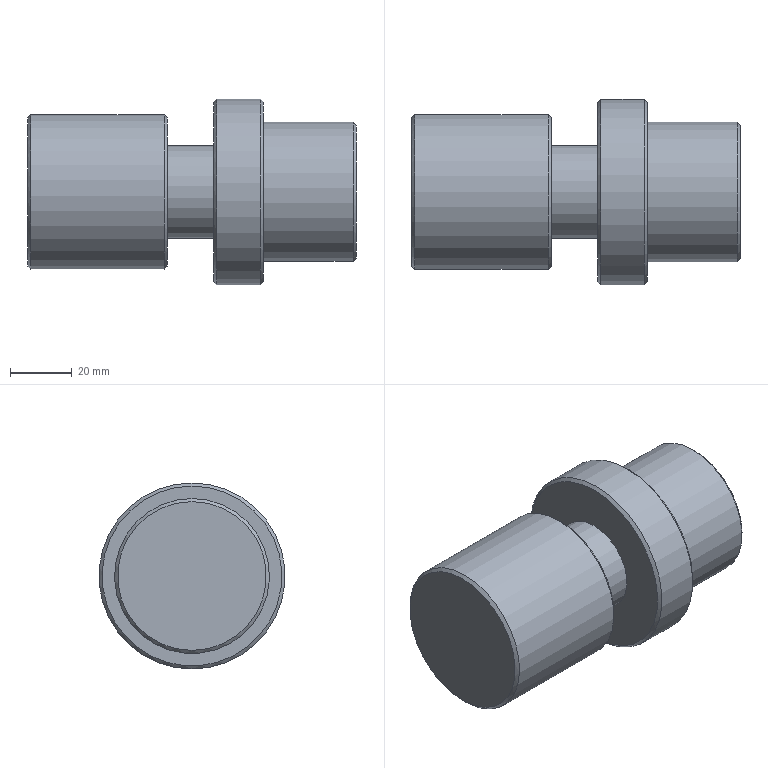Part | STEP file | Tube feed_id686_x_t | 1 solid | 14 faces | box 106 x 60 x 60 mm | volume 191501 mm3 | plane 5 | cone 5 | cylinder 4 | commonest cylinder face diameters 30 x1 45 x1 50 x1 60 x1
STEP:
#1=CARTESIAN_POINT('',(0.,0.,0.));
#2=DIRECTION('',(0.,0.,1.));
#3=DIRECTION('',(1.,0.,0.));
#4=AXIS2_PLACEMENT_3D('',#1,#2,#3);
#5=CARTESIAN_POINT('',(271.,210.936,18.5));
#6=VERTEX_POINT('',#5);
#7=CARTESIAN_POINT('',(271.,210.936,-4.));
#8=DIRECTION('',(-1.,0.,0.));
#9=DIRECTION('',(0.,0.,1.));
#10=AXIS2_PLACEMENT_3D('',#7,#8,#9);
#11=CIRCLE('',#10,22.5);
#12=CARTESIAN_POINT('',(272.,210.936,-4.));
#13=DIRECTION('',(-1.,0.,0.));
#14=DIRECTION('',(0.,0.,1.));
#15=AXIS2_PLACEMENT_3D('',#12,#13,#14);
#16=CYLINDRICAL_SURFACE('',#15,22.5);
#17=CARTESIAN_POINT('',(0.,1.));
#18=DIRECTION('',(1.,0.));
#19=VECTOR('',#18,1.);
#20=LINE('',#17,#19);
#21=(GEOMETRIC_REPRESENTATION_CONTEXT(2)PARAMETRIC_REPRESENTATION_CONTEXT()REPRESENTATION_CONTEXT('',''));
#22=DEFINITIONAL_REPRESENTATION('',(#20),#21);
#23=PCURVE('',#16,#22);
#24=CARTESIAN_POINT('',(271.,210.936,-4.));
#25=DIRECTION('',(-1.,0.,0.));
#26=DIRECTION('',(0.,0.,1.));
#27=AXIS2_PLACEMENT_3D('',#24,#25,#26);
#28=CONICAL_SURFACE('',#27,22.5,0.7854);
#29=CARTESIAN_POINT('',(0.,0.));
#30=DIRECTION('',(1.,0.));
#31=VECTOR('',#30,1.);
#32=LINE('',#29,#31);
#33=(GEOMETRIC_REPRESENTATION_CONTEXT(2)PARAMETRIC_REPRESENTATION_CONTEXT()REPRESENTATION_CONTEXT('',''));
#34=DEFINITIONAL_REPRESENTATION('',(#32),#33);
#35=PCURVE('',#28,#34);
#36=SURFACE_CURVE('',#11,(#23,#35),.PCURVE_S1.);
#37=EDGE_CURVE('',#6,#6,#36,.T.);
#38=ORIENTED_EDGE('',*,*,#37,.T.);
#39=CARTESIAN_POINT('',(242.,210.936,18.5));
#40=VERTEX_POINT('',#39);
#41=CARTESIAN_POINT('',(271.,210.936,18.5));
#42=CARTESIAN_POINT('',(242.,210.936,18.5));
#43=B_SPLINE_CURVE_WITH_KNOTS('',1,(#41,#42),.UNSPECIFIED.,.F.,.F.,(2,2),(1.,30.),.PIECEWISE_BEZIER_KNOTS.);
#44=CARTESIAN_POINT('',(6.283,0.));
#45=DIRECTION('',(0.,1.));
#46=VECTOR('',#45,1.);
#47=LINE('',#44,#46);
#48=(GEOMETRIC_REPRESENTATION_CONTEXT(2)PARAMETRIC_REPRESENTATION_CONTEXT()REPRESENTATION_CONTEXT('',''));
#49=DEFINITIONAL_REPRESENTATION('',(#47),#48);
#50=PCURVE('',#16,#49);
#51=CARTESIAN_POINT('',(0.,0.));
#52=DIRECTION('',(0.,1.));
#53=VECTOR('',#52,1.);
#54=LINE('',#51,#53);
#55=(GEOMETRIC_REPRESENTATION_CONTEXT(2)PARAMETRIC_REPRESENTATION_CONTEXT()REPRESENTATION_CONTEXT('',''));
#56=DEFINITIONAL_REPRESENTATION('',(#54),#55);
#57=PCURVE('',#16,#56);
#58=SEAM_CURVE('',#43,(#50,#57),.PCURVE_S1.);
#59=EDGE_CURVE('',#6,#40,#58,.T.);
#60=ORIENTED_EDGE('',*,*,#59,.T.);
#61=CARTESIAN_POINT('',(242.,210.936,-4.));
#62=DIRECTION('',(-1.,0.,0.));
#63=DIRECTION('',(0.,0.,1.));
#64=AXIS2_PLACEMENT_3D('',#61,#62,#63);
#65=CIRCLE('',#64,22.5);
#66=CARTESIAN_POINT('',(0.,30.));
#67=DIRECTION('',(1.,0.));
#68=VECTOR('',#67,1.);
#69=LINE('',#66,#68);
#70=(GEOMETRIC_REPRESENTATION_CONTEXT(2)PARAMETRIC_REPRESENTATION_CONTEXT()REPRESENTATION_CONTEXT('',''));
#71=DEFINITIONAL_REPRESENTATION('',(#69),#70);
#72=PCURVE('',#16,#71);
#73=CARTESIAN_POINT('',(242.,210.936,-4.));
#74=DIRECTION('',(-1.,0.,0.));
#75=DIRECTION('',(0.,0.,1.));
#76=AXIS2_PLACEMENT_3D('',#73,#74,#75);
#77=PLANE('',#76);
#78=CARTESIAN_POINT('',(0.,0.));
#79=DIRECTION('',(1.,0.));
#80=AXIS2_PLACEMENT_2D('',#78,#79);
#81=CIRCLE('',#80,22.5);
#82=(GEOMETRIC_REPRESENTATION_CONTEXT(2)PARAMETRIC_REPRESENTATION_CONTEXT()REPRESENTATION_CONTEXT('',''));
#83=DEFINITIONAL_REPRESENTATION('',(#81),#82);
#84=PCURVE('',#77,#83);
#85=SURFACE_CURVE('',#65,(#72,#84),.PCURVE_S1.);
#86=EDGE_CURVE('',#40,#40,#85,.T.);
#87=ORIENTED_EDGE('',*,*,#86,.F.);
#88=ORIENTED_EDGE('',*,*,#59,.F.);
#89=EDGE_LOOP('',(#38,#60,#87,#88));
#90=FACE_BOUND('',#89,.T.);
#91=ADVANCED_FACE('',(#90),#16,.T.);
#92=CARTESIAN_POINT('',(272.,210.936,17.5));
#93=VERTEX_POINT('',#92);
#94=CARTESIAN_POINT('',(272.,210.936,-4.));
#95=DIRECTION('',(1.,0.,0.));
#96=DIRECTION('',(0.,0.,1.));
#97=AXIS2_PLACEMENT_3D('',#94,#95,#96);
#98=CIRCLE('',#97,21.5);
#99=CARTESIAN_POINT('',(272.,210.936,-4.));
#100=DIRECTION('',(-1.,0.,0.));
#101=DIRECTION('',(0.,0.,1.));
#102=AXIS2_PLACEMENT_3D('',#99,#100,#101);
#103=PLANE('',#102);
#104=CARTESIAN_POINT('',(21.5,0.));
#105=CARTESIAN_POINT('',(21.5,-37.239));
#106=CARTESIAN_POINT('',(-10.75,-18.62));
#107=CARTESIAN_POINT('',(-43.,0.));
#108=CARTESIAN_POINT('',(-10.75,18.62));
#109=CARTESIAN_POINT('',(21.5,37.239));
#110=CARTESIAN_POINT('',(21.5,0.));
#111=(BOUNDED_CURVE()B_SPLINE_CURVE(2,(#104,#105,#106,#107,#108,#109,#110),.UNSPECIFIED.,.T.,.F.)B_SPLINE_CURVE_WITH_KNOTS((1,2,2,2,2,1),(-2.094,0.,2.094,4.189,6.283,8.378),.UNSPECIFIED.)CURVE()GEOMETRIC_REPRESENTATION_ITEM()RATIONAL_B_SPLINE_CURVE((1.,0.5,1.,0.5,1.,0.5,1.))REPRESENTATION_ITEM(''));
#112=(GEOMETRIC_REPRESENTATION_CONTEXT(2)PARAMETRIC_REPRESENTATION_CONTEXT()REPRESENTATION_CONTEXT('',''));
#113=DEFINITIONAL_REPRESENTATION('',(#111),#112);
#114=PCURVE('',#103,#113);
#115=CARTESIAN_POINT('',(6.283,-1.));
#116=DIRECTION('',(-1.,0.));
#117=VECTOR('',#116,1.);
#118=LINE('',#115,#117);
#119=(GEOMETRIC_REPRESENTATION_CONTEXT(2)PARAMETRIC_REPRESENTATION_CONTEXT()REPRESENTATION_CONTEXT('',''));
#120=DEFINITIONAL_REPRESENTATION('',(#118),#119);
#121=PCURVE('',#28,#120);
#122=SURFACE_CURVE('',#98,(#114,#121),.PCURVE_S1.);
#123=EDGE_CURVE('',#93,#93,#122,.T.);
#124=ORIENTED_EDGE('',*,*,#123,.T.);
#125=EDGE_LOOP('',(#124));
#126=FACE_BOUND('',#125,.T.);
#127=ADVANCED_FACE('',(#126),#103,.F.);
#128=CARTESIAN_POINT('',(241.,210.936,26.));
#129=VERTEX_POINT('',#128);
#130=CARTESIAN_POINT('',(241.,210.936,-4.));
#131=DIRECTION('',(-1.,0.,0.));
#132=DIRECTION('',(0.,0.,1.));
#133=AXIS2_PLACEMENT_3D('',#130,#131,#132);
#134=CIRCLE('',#133,30.);
#135=CARTESIAN_POINT('',(232.,210.936,-4.));
#136=DIRECTION('',(1.,0.,0.));
#137=DIRECTION('',(0.,0.,-1.));
#138=AXIS2_PLACEMENT_3D('',#135,#136,#137);
#139=CYLINDRICAL_SURFACE('',#138,30.);
#140=CARTESIAN_POINT('',(9.425,9.));
#141=DIRECTION('',(-1.,0.));
#142=VECTOR('',#141,1.);
#143=LINE('',#140,#142);
#144=(GEOMETRIC_REPRESENTATION_CONTEXT(2)PARAMETRIC_REPRESENTATION_CONTEXT()REPRESENTATION_CONTEXT('',''));
#145=DEFINITIONAL_REPRESENTATION('',(#143),#144);
#146=PCURVE('',#139,#145);
#147=CARTESIAN_POINT('',(241.,210.936,-4.));
#148=DIRECTION('',(-1.,0.,0.));
#149=DIRECTION('',(0.,0.,1.));
#150=AXIS2_PLACEMENT_3D('',#147,#148,#149);
#151=CONICAL_SURFACE('',#150,30.,0.7854);
#152=CARTESIAN_POINT('',(0.,0.));
#153=DIRECTION('',(1.,0.));
#154=VECTOR('',#153,1.);
#155=LINE('',#152,#154);
#156=(GEOMETRIC_REPRESENTATION_CONTEXT(2)PARAMETRIC_REPRESENTATION_CONTEXT()REPRESENTATION_CONTEXT('',''));
#157=DEFINITIONAL_REPRESENTATION('',(#155),#156);
#158=PCURVE('',#151,#157);
#159=SURFACE_CURVE('',#134,(#146,#158),.PCURVE_S1.);
#160=EDGE_CURVE('',#129,#129,#159,.T.);
#161=ORIENTED_EDGE('',*,*,#160,.T.);
#162=CARTESIAN_POINT('',(227.,210.936,26.));
#163=VERTEX_POINT('',#162);
#164=CARTESIAN_POINT('',(227.,210.936,26.));
#165=CARTESIAN_POINT('',(241.,210.936,26.));
#166=B_SPLINE_CURVE_WITH_KNOTS('',1,(#164,#165),.UNSPECIFIED.,.F.,.F.,(2,2),(-5.,9.),.PIECEWISE_BEZIER_KNOTS.);
#167=CARTESIAN_POINT('',(3.142,0.));
#168=DIRECTION('',(0.,1.));
#169=VECTOR('',#168,1.);
#170=LINE('',#167,#169);
#171=(GEOMETRIC_REPRESENTATION_CONTEXT(2)PARAMETRIC_REPRESENTATION_CONTEXT()REPRESENTATION_CONTEXT('',''));
#172=DEFINITIONAL_REPRESENTATION('',(#170),#171);
#173=PCURVE('',#139,#172);
#174=CARTESIAN_POINT('',(9.425,0.));
#175=DIRECTION('',(0.,1.));
#176=VECTOR('',#175,1.);
#177=LINE('',#174,#176);
#178=(GEOMETRIC_REPRESENTATION_CONTEXT(2)PARAMETRIC_REPRESENTATION_CONTEXT()REPRESENTATION_CONTEXT('',''));
#179=DEFINITIONAL_REPRESENTATION('',(#177),#178);
#180=PCURVE('',#139,#179);
#181=SEAM_CURVE('',#166,(#173,#180),.PCURVE_S1.);
#182=EDGE_CURVE('',#163,#129,#181,.T.);
#183=ORIENTED_EDGE('',*,*,#182,.F.);
#184=CARTESIAN_POINT('',(227.,210.936,-4.));
#185=DIRECTION('',(1.,0.,0.));
#186=DIRECTION('',(0.,0.,1.));
#187=AXIS2_PLACEMENT_3D('',#184,#185,#186);
#188=CIRCLE('',#187,30.);
#189=CARTESIAN_POINT('',(3.142,-5.));
#190=DIRECTION('',(1.,0.));
#191=VECTOR('',#190,1.);
#192=LINE('',#189,#191);
#193=(GEOMETRIC_REPRESENTATION_CONTEXT(2)PARAMETRIC_REPRESENTATION_CONTEXT()REPRESENTATION_CONTEXT('',''));
#194=DEFINITIONAL_REPRESENTATION('',(#192),#193);
#195=PCURVE('',#139,#194);
#196=CARTESIAN_POINT('',(226.,210.936,-4.));
#197=DIRECTION('',(1.,0.,0.));
#198=DIRECTION('',(0.,0.,-1.));
#199=AXIS2_PLACEMENT_3D('',#196,#197,#198);
#200=CONICAL_SURFACE('',#199,29.,0.7854);
#201=CARTESIAN_POINT('',(3.142,1.));
#202=DIRECTION('',(1.,0.));
#203=VECTOR('',#202,1.);
#204=LINE('',#201,#203);
#205=(GEOMETRIC_REPRESENTATION_CONTEXT(2)PARAMETRIC_REPRESENTATION_CONTEXT()REPRESENTATION_CONTEXT('',''));
#206=DEFINITIONAL_REPRESENTATION('',(#204),#205);
#207=PCURVE('',#200,#206);
#208=SURFACE_CURVE('',#188,(#195,#207),.PCURVE_S1.);
#209=EDGE_CURVE('',#163,#163,#208,.T.);
#210=ORIENTED_EDGE('',*,*,#209,.T.);
#211=ORIENTED_EDGE('',*,*,#182,.T.);
#212=EDGE_LOOP('',(#161,#183,#210,#211));
#213=FACE_BOUND('',#212,.T.);
#214=ADVANCED_FACE('',(#213),#139,.T.);
#215=CARTESIAN_POINT('',(226.,210.936,25.));
#216=VERTEX_POINT('',#215);
#217=CARTESIAN_POINT('',(226.,210.936,-4.));
#218=DIRECTION('',(-1.,0.,0.));
#219=DIRECTION('',(0.,0.,1.));
#220=AXIS2_PLACEMENT_3D('',#217,#218,#219);
#221=CIRCLE('',#220,29.);
#222=CARTESIAN_POINT('',(226.,160.936,14.));
#223=DIRECTION('',(-1.,0.,0.));
#224=DIRECTION('',(0.,0.,1.));
#225=AXIS2_PLACEMENT_3D('',#222,#223,#224);
#226=PLANE('',#225);
#227=CARTESIAN_POINT('',(-18.,50.));
#228=DIRECTION('',(1.,0.));
#229=AXIS2_PLACEMENT_2D('',#227,#228);
#230=CIRCLE('',#229,29.);
#231=(GEOMETRIC_REPRESENTATION_CONTEXT(2)PARAMETRIC_REPRESENTATION_CONTEXT()REPRESENTATION_CONTEXT('',''));
#232=DEFINITIONAL_REPRESENTATION('',(#230),#231);
#233=PCURVE('',#226,#232);
#234=CARTESIAN_POINT('',(9.425,0.));
#235=DIRECTION('',(-1.,0.));
#236=VECTOR('',#235,1.);
#237=LINE('',#234,#236);
#238=(GEOMETRIC_REPRESENTATION_CONTEXT(2)PARAMETRIC_REPRESENTATION_CONTEXT()REPRESENTATION_CONTEXT('',''));
#239=DEFINITIONAL_REPRESENTATION('',(#237),#238);
#240=PCURVE('',#200,#239);
#241=SURFACE_CURVE('',#221,(#233,#240),.PCURVE_S1.);
#242=EDGE_CURVE('',#216,#216,#241,.T.);
#243=ORIENTED_EDGE('',*,*,#242,.T.);
#244=EDGE_LOOP('',(#243));
#245=FACE_BOUND('',#244,.T.);
#246=CARTESIAN_POINT('',(226.,210.936,11.));
#247=VERTEX_POINT('',#246);
#248=CARTESIAN_POINT('',(226.,210.936,-4.));
#249=DIRECTION('',(-1.,0.,0.));
#250=DIRECTION('',(0.,0.,1.));
#251=AXIS2_PLACEMENT_3D('',#248,#249,#250);
#252=CIRCLE('',#251,15.);
#253=CARTESIAN_POINT('',(-18.,50.));
#254=DIRECTION('',(1.,0.));
#255=AXIS2_PLACEMENT_2D('',#253,#254);
#256=CIRCLE('',#255,15.);
#257=(GEOMETRIC_REPRESENTATION_CONTEXT(2)PARAMETRIC_REPRESENTATION_CONTEXT()REPRESENTATION_CONTEXT('',''));
#258=DEFINITIONAL_REPRESENTATION('',(#256),#257);
#259=PCURVE('',#226,#258);
#260=CARTESIAN_POINT('',(211.,210.936,-4.));
#261=DIRECTION('',(1.,0.,0.));
#262=DIRECTION('',(0.,0.,-1.));
#263=AXIS2_PLACEMENT_3D('',#260,#261,#262);
#264=CYLINDRICAL_SURFACE('',#263,15.);
#265=CARTESIAN_POINT('',(9.425,15.));
#266=DIRECTION('',(-1.,0.));
#267=VECTOR('',#266,1.);
#268=LINE('',#265,#267);
#269=(GEOMETRIC_REPRESENTATION_CONTEXT(2)PARAMETRIC_REPRESENTATION_CONTEXT()REPRESENTATION_CONTEXT('',''));
#270=DEFINITIONAL_REPRESENTATION('',(#268),#269);
#271=PCURVE('',#264,#270);
#272=SURFACE_CURVE('',#252,(#259,#271),.PCURVE_S1.);
#273=EDGE_CURVE('',#247,#247,#272,.T.);
#274=ORIENTED_EDGE('',*,*,#273,.F.);
#275=EDGE_LOOP('',(#274));
#276=FACE_BOUND('',#275,.T.);
#277=ADVANCED_FACE('',(#245,#276),#226,.T.);
#278=CARTESIAN_POINT('',(242.,210.936,25.));
#279=VERTEX_POINT('',#278);
#280=CARTESIAN_POINT('',(242.,210.936,-4.));
#281=DIRECTION('',(1.,0.,0.));
#282=DIRECTION('',(0.,0.,1.));
#283=AXIS2_PLACEMENT_3D('',#280,#281,#282);
#284=CIRCLE('',#283,29.);
#285=CARTESIAN_POINT('',(29.,0.));
#286=CARTESIAN_POINT('',(29.,-50.229));
#287=CARTESIAN_POINT('',(-14.5,-25.115));
#288=CARTESIAN_POINT('',(-58.,0.));
#289=CARTESIAN_POINT('',(-14.5,25.115));
#290=CARTESIAN_POINT('',(29.,50.229));
#291=CARTESIAN_POINT('',(29.,0.));
#292=(BOUNDED_CURVE()B_SPLINE_CURVE(2,(#285,#286,#287,#288,#289,#290,#291),.UNSPECIFIED.,.T.,.F.)B_SPLINE_CURVE_WITH_KNOTS((1,2,2,2,2,1),(-2.094,0.,2.094,4.189,6.283,8.378),.UNSPECIFIED.)CURVE()GEOMETRIC_REPRESENTATION_ITEM()RATIONAL_B_SPLINE_CURVE((1.,0.5,1.,0.5,1.,0.5,1.))REPRESENTATION_ITEM(''));
#293=(GEOMETRIC_REPRESENTATION_CONTEXT(2)PARAMETRIC_REPRESENTATION_CONTEXT()REPRESENTATION_CONTEXT('',''));
#294=DEFINITIONAL_REPRESENTATION('',(#292),#293);
#295=PCURVE('',#77,#294);
#296=CARTESIAN_POINT('',(6.283,-1.));
#297=DIRECTION('',(-1.,0.));
#298=VECTOR('',#297,1.);
#299=LINE('',#296,#298);
#300=(GEOMETRIC_REPRESENTATION_CONTEXT(2)PARAMETRIC_REPRESENTATION_CONTEXT()REPRESENTATION_CONTEXT('',''));
#301=DEFINITIONAL_REPRESENTATION('',(#299),#300);
#302=PCURVE('',#151,#301);
#303=SURFACE_CURVE('',#284,(#295,#302),.PCURVE_S1.);
#304=EDGE_CURVE('',#279,#279,#303,.T.);
#305=ORIENTED_EDGE('',*,*,#304,.T.);
#306=EDGE_LOOP('',(#305));
#307=FACE_BOUND('',#306,.T.);
#308=ORIENTED_EDGE('',*,*,#86,.T.);
#309=EDGE_LOOP('',(#308));
#310=FACE_BOUND('',#309,.T.);
#311=ADVANCED_FACE('',(#307,#310),#77,.F.);
#312=CARTESIAN_POINT('',(210.,210.936,21.));
#313=VERTEX_POINT('',#312);
#314=CARTESIAN_POINT('',(210.,210.936,-4.));
#315=DIRECTION('',(-1.,0.,0.));
#316=DIRECTION('',(0.,0.,1.));
#317=AXIS2_PLACEMENT_3D('',#314,#315,#316);
#318=CIRCLE('',#317,25.);
#319=CARTESIAN_POINT('',(211.,210.936,-4.));
#320=DIRECTION('',(-1.,0.,0.));
#321=DIRECTION('',(0.,0.,1.));
#322=AXIS2_PLACEMENT_3D('',#319,#320,#321);
#323=CYLINDRICAL_SURFACE('',#322,25.);
#324=CARTESIAN_POINT('',(0.,1.));
#325=DIRECTION('',(1.,0.));
#326=VECTOR('',#325,1.);
#327=LINE('',#324,#326);
#328=(GEOMETRIC_REPRESENTATION_CONTEXT(2)PARAMETRIC_REPRESENTATION_CONTEXT()REPRESENTATION_CONTEXT('',''));
#329=DEFINITIONAL_REPRESENTATION('',(#327),#328);
#330=PCURVE('',#323,#329);
#331=CARTESIAN_POINT('',(210.,210.936,-4.));
#332=DIRECTION('',(-1.,0.,0.));
#333=DIRECTION('',(0.,0.,1.));
#334=AXIS2_PLACEMENT_3D('',#331,#332,#333);
#335=CONICAL_SURFACE('',#334,25.,0.7854);
#336=CARTESIAN_POINT('',(0.,0.));
#337=DIRECTION('',(1.,0.));
#338=VECTOR('',#337,1.);
#339=LINE('',#336,#338);
#340=(GEOMETRIC_REPRESENTATION_CONTEXT(2)PARAMETRIC_REPRESENTATION_CONTEXT()REPRESENTATION_CONTEXT('',''));
#341=DEFINITIONAL_REPRESENTATION('',(#339),#340);
#342=PCURVE('',#335,#341);
#343=SURFACE_CURVE('',#318,(#330,#342),.PCURVE_S1.);
#344=EDGE_CURVE('',#313,#313,#343,.T.);
#345=ORIENTED_EDGE('',*,*,#344,.T.);
#346=CARTESIAN_POINT('',(167.,210.936,21.));
#347=VERTEX_POINT('',#346);
#348=CARTESIAN_POINT('',(210.,210.936,21.));
#349=CARTESIAN_POINT('',(167.,210.936,21.));
#350=B_SPLINE_CURVE_WITH_KNOTS('',1,(#348,#349),.UNSPECIFIED.,.F.,.F.,(2,2),(1.,44.),.PIECEWISE_BEZIER_KNOTS.);
#351=CARTESIAN_POINT('',(6.283,0.));
#352=DIRECTION('',(0.,1.));
#353=VECTOR('',#352,1.);
#354=LINE('',#351,#353);
#355=(GEOMETRIC_REPRESENTATION_CONTEXT(2)PARAMETRIC_REPRESENTATION_CONTEXT()REPRESENTATION_CONTEXT('',''));
#356=DEFINITIONAL_REPRESENTATION('',(#354),#355);
#357=PCURVE('',#323,#356);
#358=CARTESIAN_POINT('',(0.,0.));
#359=DIRECTION('',(0.,1.));
#360=VECTOR('',#359,1.);
#361=LINE('',#358,#360);
#362=(GEOMETRIC_REPRESENTATION_CONTEXT(2)PARAMETRIC_REPRESENTATION_CONTEXT()REPRESENTATION_CONTEXT('',''));
#363=DEFINITIONAL_REPRESENTATION('',(#361),#362);
#364=PCURVE('',#323,#363);
#365=SEAM_CURVE('',#350,(#357,#364),.PCURVE_S1.);
#366=EDGE_CURVE('',#313,#347,#365,.T.);
#367=ORIENTED_EDGE('',*,*,#366,.T.);
#368=CARTESIAN_POINT('',(167.,210.936,-4.));
#369=DIRECTION('',(1.,0.,0.));
#370=DIRECTION('',(0.,0.,1.));
#371=AXIS2_PLACEMENT_3D('',#368,#369,#370);
#372=CIRCLE('',#371,25.);
#373=CARTESIAN_POINT('',(6.283,44.));
#374=DIRECTION('',(-1.,0.));
#375=VECTOR('',#374,1.);
#376=LINE('',#373,#375);
#377=(GEOMETRIC_REPRESENTATION_CONTEXT(2)PARAMETRIC_REPRESENTATION_CONTEXT()REPRESENTATION_CONTEXT('',''));
#378=DEFINITIONAL_REPRESENTATION('',(#376),#377);
#379=PCURVE('',#323,#378);
#380=CARTESIAN_POINT('',(166.,210.936,-4.));
#381=DIRECTION('',(1.,0.,0.));
#382=DIRECTION('',(0.,0.,-1.));
#383=AXIS2_PLACEMENT_3D('',#380,#381,#382);
#384=CONICAL_SURFACE('',#383,24.,0.7854);
#385=CARTESIAN_POINT('',(3.142,1.));
#386=DIRECTION('',(1.,0.));
#387=VECTOR('',#386,1.);
#388=LINE('',#385,#387);
#389=(GEOMETRIC_REPRESENTATION_CONTEXT(2)PARAMETRIC_REPRESENTATION_CONTEXT()REPRESENTATION_CONTEXT('',''));
#390=DEFINITIONAL_REPRESENTATION('',(#388),#389);
#391=PCURVE('',#384,#390);
#392=SURFACE_CURVE('',#372,(#379,#391),.PCURVE_S1.);
#393=EDGE_CURVE('',#347,#347,#392,.T.);
#394=ORIENTED_EDGE('',*,*,#393,.T.);
#395=ORIENTED_EDGE('',*,*,#366,.F.);
#396=EDGE_LOOP('',(#345,#367,#394,#395));
#397=FACE_BOUND('',#396,.T.);
#398=ADVANCED_FACE('',(#397),#323,.T.);
#399=CARTESIAN_POINT('',(211.,210.936,20.));
#400=VERTEX_POINT('',#399);
#401=CARTESIAN_POINT('',(211.,210.936,-4.));
#402=DIRECTION('',(1.,0.,0.));
#403=DIRECTION('',(0.,0.,1.));
#404=AXIS2_PLACEMENT_3D('',#401,#402,#403);
#405=CIRCLE('',#404,24.);
#406=CARTESIAN_POINT('',(211.,210.936,-4.));
#407=DIRECTION('',(-1.,0.,0.));
#408=DIRECTION('',(0.,0.,1.));
#409=AXIS2_PLACEMENT_3D('',#406,#407,#408);
#410=PLANE('',#409);
#411=CARTESIAN_POINT('',(24.,0.));
#412=CARTESIAN_POINT('',(24.,-41.569));
#413=CARTESIAN_POINT('',(-12.,-20.785));
#414=CARTESIAN_POINT('',(-48.,0.));
#415=CARTESIAN_POINT('',(-12.,20.785));
#416=CARTESIAN_POINT('',(24.,41.569));
#417=CARTESIAN_POINT('',(24.,0.));
#418=(BOUNDED_CURVE()B_SPLINE_CURVE(2,(#411,#412,#413,#414,#415,#416,#417),.UNSPECIFIED.,.T.,.F.)B_SPLINE_CURVE_WITH_KNOTS((1,2,2,2,2,1),(-2.094,0.,2.094,4.189,6.283,8.378),.UNSPECIFIED.)CURVE()GEOMETRIC_REPRESENTATION_ITEM()RATIONAL_B_SPLINE_CURVE((1.,0.5,1.,0.5,1.,0.5,1.))REPRESENTATION_ITEM(''));
#419=(GEOMETRIC_REPRESENTATION_CONTEXT(2)PARAMETRIC_REPRESENTATION_CONTEXT()REPRESENTATION_CONTEXT('',''));
#420=DEFINITIONAL_REPRESENTATION('',(#418),#419);
#421=PCURVE('',#410,#420);
#422=CARTESIAN_POINT('',(6.283,-1.));
#423=DIRECTION('',(-1.,0.));
#424=VECTOR('',#423,1.);
#425=LINE('',#422,#424);
#426=(GEOMETRIC_REPRESENTATION_CONTEXT(2)PARAMETRIC_REPRESENTATION_CONTEXT()REPRESENTATION_CONTEXT('',''));
#427=DEFINITIONAL_REPRESENTATION('',(#425),#426);
#428=PCURVE('',#335,#427);
#429=SURFACE_CURVE('',#405,(#421,#428),.PCURVE_S1.);
#430=EDGE_CURVE('',#400,#400,#429,.T.);
#431=ORIENTED_EDGE('',*,*,#430,.T.);
#432=EDGE_LOOP('',(#431));
#433=FACE_BOUND('',#432,.T.);
#434=CARTESIAN_POINT('',(211.,210.936,11.));
#435=VERTEX_POINT('',#434);
#436=CARTESIAN_POINT('',(211.,210.936,-4.));
#437=DIRECTION('',(-1.,0.,0.));
#438=DIRECTION('',(0.,0.,1.));
#439=AXIS2_PLACEMENT_3D('',#436,#437,#438);
#440=CIRCLE('',#439,15.);
#441=CARTESIAN_POINT('',(0.,0.));
#442=DIRECTION('',(1.,0.));
#443=AXIS2_PLACEMENT_2D('',#441,#442);
#444=CIRCLE('',#443,15.);
#445=(GEOMETRIC_REPRESENTATION_CONTEXT(2)PARAMETRIC_REPRESENTATION_CONTEXT()REPRESENTATION_CONTEXT('',''));
#446=DEFINITIONAL_REPRESENTATION('',(#444),#445);
#447=PCURVE('',#410,#446);
#448=CARTESIAN_POINT('',(9.425,0.));
#449=DIRECTION('',(-1.,0.));
#450=VECTOR('',#449,1.);
#451=LINE('',#448,#450);
#452=(GEOMETRIC_REPRESENTATION_CONTEXT(2)PARAMETRIC_REPRESENTATION_CONTEXT()REPRESENTATION_CONTEXT('',''));
#453=DEFINITIONAL_REPRESENTATION('',(#451),#452);
#454=PCURVE('',#264,#453);
#455=SURFACE_CURVE('',#440,(#447,#454),.PCURVE_S1.);
#456=EDGE_CURVE('',#435,#435,#455,.T.);
#457=ORIENTED_EDGE('',*,*,#456,.T.);
#458=EDGE_LOOP('',(#457));
#459=FACE_BOUND('',#458,.T.);
#460=ADVANCED_FACE('',(#433,#459),#410,.F.);
#461=CARTESIAN_POINT('',(166.,210.936,20.));
#462=VERTEX_POINT('',#461);
#463=CARTESIAN_POINT('',(166.,210.936,-4.));
#464=DIRECTION('',(-1.,0.,0.));
#465=DIRECTION('',(0.,0.,1.));
#466=AXIS2_PLACEMENT_3D('',#463,#464,#465);
#467=CIRCLE('',#466,24.);
#468=CARTESIAN_POINT('',(166.,210.936,-4.));
#469=DIRECTION('',(-1.,0.,0.));
#470=DIRECTION('',(0.,0.,1.));
#471=AXIS2_PLACEMENT_3D('',#468,#469,#470);
#472=PLANE('',#471);
#473=CARTESIAN_POINT('',(0.,0.));
#474=DIRECTION('',(1.,0.));
#475=AXIS2_PLACEMENT_2D('',#473,#474);
#476=CIRCLE('',#475,24.);
#477=(GEOMETRIC_REPRESENTATION_CONTEXT(2)PARAMETRIC_REPRESENTATION_CONTEXT()REPRESENTATION_CONTEXT('',''));
#478=DEFINITIONAL_REPRESENTATION('',(#476),#477);
#479=PCURVE('',#472,#478);
#480=CARTESIAN_POINT('',(9.425,0.));
#481=DIRECTION('',(-1.,0.));
#482=VECTOR('',#481,1.);
#483=LINE('',#480,#482);
#484=(GEOMETRIC_REPRESENTATION_CONTEXT(2)PARAMETRIC_REPRESENTATION_CONTEXT()REPRESENTATION_CONTEXT('',''));
#485=DEFINITIONAL_REPRESENTATION('',(#483),#484);
#486=PCURVE('',#384,#485);
#487=SURFACE_CURVE('',#467,(#479,#486),.PCURVE_S1.);
#488=EDGE_CURVE('',#462,#462,#487,.T.);
#489=ORIENTED_EDGE('',*,*,#488,.T.);
#490=EDGE_LOOP('',(#489));
#491=FACE_BOUND('',#490,.T.);
#492=ADVANCED_FACE('',(#491),#472,.T.);
#493=ORIENTED_EDGE('',*,*,#456,.F.);
#494=CARTESIAN_POINT('',(211.,210.936,11.));
#495=CARTESIAN_POINT('',(226.,210.936,11.));
#496=B_SPLINE_CURVE_WITH_KNOTS('',1,(#494,#495),.UNSPECIFIED.,.F.,.F.,(2,2),(0.,15.),.PIECEWISE_BEZIER_KNOTS.);
#497=CARTESIAN_POINT('',(9.425,0.));
#498=DIRECTION('',(0.,1.));
#499=VECTOR('',#498,1.);
#500=LINE('',#497,#499);
#501=(GEOMETRIC_REPRESENTATION_CONTEXT(2)PARAMETRIC_REPRESENTATION_CONTEXT()REPRESENTATION_CONTEXT('',''));
#502=DEFINITIONAL_REPRESENTATION('',(#500),#501);
#503=PCURVE('',#264,#502);
#504=CARTESIAN_POINT('',(3.142,0.));
#505=DIRECTION('',(0.,1.));
#506=VECTOR('',#505,1.);
#507=LINE('',#504,#506);
#508=(GEOMETRIC_REPRESENTATION_CONTEXT(2)PARAMETRIC_REPRESENTATION_CONTEXT()REPRESENTATION_CONTEXT('',''));
#509=DEFINITIONAL_REPRESENTATION('',(#507),#508);
#510=PCURVE('',#264,#509);
#511=SEAM_CURVE('',#496,(#503,#510),.PCURVE_S1.);
#512=EDGE_CURVE('',#435,#247,#511,.T.);
#513=ORIENTED_EDGE('',*,*,#512,.T.);
#514=ORIENTED_EDGE('',*,*,#273,.T.);
#515=ORIENTED_EDGE('',*,*,#512,.F.);
#516=EDGE_LOOP('',(#493,#513,#514,#515));
#517=FACE_BOUND('',#516,.T.);
#518=ADVANCED_FACE('',(#517),#264,.T.);
#519=ORIENTED_EDGE('',*,*,#123,.F.);
#520=CARTESIAN_POINT('',(272.,210.936,17.5));
#521=CARTESIAN_POINT('',(271.,210.936,18.5));
#522=B_SPLINE_CURVE_WITH_KNOTS('',1,(#520,#521),.UNSPECIFIED.,.F.,.F.,(2,2),(-1.414,0.),.PIECEWISE_BEZIER_KNOTS.);
#523=CARTESIAN_POINT('',(6.283,0.));
#524=DIRECTION('',(0.,1.));
#525=VECTOR('',#524,1.);
#526=LINE('',#523,#525);
#527=(GEOMETRIC_REPRESENTATION_CONTEXT(2)PARAMETRIC_REPRESENTATION_CONTEXT()REPRESENTATION_CONTEXT('',''));
#528=DEFINITIONAL_REPRESENTATION('',(#526),#527);
#529=PCURVE('',#28,#528);
#530=CARTESIAN_POINT('',(0.,0.));
#531=DIRECTION('',(0.,1.));
#532=VECTOR('',#531,1.);
#533=LINE('',#530,#532);
#534=(GEOMETRIC_REPRESENTATION_CONTEXT(2)PARAMETRIC_REPRESENTATION_CONTEXT()REPRESENTATION_CONTEXT('',''));
#535=DEFINITIONAL_REPRESENTATION('',(#533),#534);
#536=PCURVE('',#28,#535);
#537=SEAM_CURVE('',#522,(#529,#536),.PCURVE_S1.);
#538=EDGE_CURVE('',#93,#6,#537,.T.);
#539=ORIENTED_EDGE('',*,*,#538,.T.);
#540=ORIENTED_EDGE('',*,*,#37,.F.);
#541=ORIENTED_EDGE('',*,*,#538,.F.);
#542=EDGE_LOOP('',(#519,#539,#540,#541));
#543=FACE_BOUND('',#542,.T.);
#544=ADVANCED_FACE('',(#543),#28,.T.);
#545=ORIENTED_EDGE('',*,*,#304,.F.);
#546=CARTESIAN_POINT('',(242.,210.936,25.));
#547=CARTESIAN_POINT('',(241.,210.936,26.));
#548=B_SPLINE_CURVE_WITH_KNOTS('',1,(#546,#547),.UNSPECIFIED.,.F.,.F.,(2,2),(-1.414,0.),.PIECEWISE_BEZIER_KNOTS.);
#549=CARTESIAN_POINT('',(6.283,0.));
#550=DIRECTION('',(0.,1.));
#551=VECTOR('',#550,1.);
#552=LINE('',#549,#551);
#553=(GEOMETRIC_REPRESENTATION_CONTEXT(2)PARAMETRIC_REPRESENTATION_CONTEXT()REPRESENTATION_CONTEXT('',''));
#554=DEFINITIONAL_REPRESENTATION('',(#552),#553);
#555=PCURVE('',#151,#554);
#556=CARTESIAN_POINT('',(0.,0.));
#557=DIRECTION('',(0.,1.));
#558=VECTOR('',#557,1.);
#559=LINE('',#556,#558);
#560=(GEOMETRIC_REPRESENTATION_CONTEXT(2)PARAMETRIC_REPRESENTATION_CONTEXT()REPRESENTATION_CONTEXT('',''));
#561=DEFINITIONAL_REPRESENTATION('',(#559),#560);
#562=PCURVE('',#151,#561);
#563=SEAM_CURVE('',#548,(#555,#562),.PCURVE_S1.);
#564=EDGE_CURVE('',#279,#129,#563,.T.);
#565=ORIENTED_EDGE('',*,*,#564,.T.);
#566=ORIENTED_EDGE('',*,*,#160,.F.);
#567=ORIENTED_EDGE('',*,*,#564,.F.);
#568=EDGE_LOOP('',(#545,#565,#566,#567));
#569=FACE_BOUND('',#568,.T.);
#570=ADVANCED_FACE('',(#569),#151,.T.);
#571=ORIENTED_EDGE('',*,*,#209,.F.);
#572=CARTESIAN_POINT('',(226.,210.936,25.));
#573=CARTESIAN_POINT('',(227.,210.936,26.));
#574=B_SPLINE_CURVE_WITH_KNOTS('',1,(#572,#573),.UNSPECIFIED.,.F.,.F.,(2,2),(0.,1.414),.PIECEWISE_BEZIER_KNOTS.);
#575=CARTESIAN_POINT('',(3.142,0.));
#576=DIRECTION('',(0.,1.));
#577=VECTOR('',#576,1.);
#578=LINE('',#575,#577);
#579=(GEOMETRIC_REPRESENTATION_CONTEXT(2)PARAMETRIC_REPRESENTATION_CONTEXT()REPRESENTATION_CONTEXT('',''));
#580=DEFINITIONAL_REPRESENTATION('',(#578),#579);
#581=PCURVE('',#200,#580);
#582=CARTESIAN_POINT('',(9.425,0.));
#583=DIRECTION('',(0.,1.));
#584=VECTOR('',#583,1.);
#585=LINE('',#582,#584);
#586=(GEOMETRIC_REPRESENTATION_CONTEXT(2)PARAMETRIC_REPRESENTATION_CONTEXT()REPRESENTATION_CONTEXT('',''));
#587=DEFINITIONAL_REPRESENTATION('',(#585),#586);
#588=PCURVE('',#200,#587);
#589=SEAM_CURVE('',#574,(#581,#588),.PCURVE_S1.);
#590=EDGE_CURVE('',#216,#163,#589,.T.);
#591=ORIENTED_EDGE('',*,*,#590,.F.);
#592=ORIENTED_EDGE('',*,*,#242,.F.);
#593=ORIENTED_EDGE('',*,*,#590,.T.);
#594=EDGE_LOOP('',(#571,#591,#592,#593));
#595=FACE_BOUND('',#594,.T.);
#596=ADVANCED_FACE('',(#595),#200,.T.);
#597=ORIENTED_EDGE('',*,*,#430,.F.);
#598=CARTESIAN_POINT('',(211.,210.936,20.));
#599=CARTESIAN_POINT('',(210.,210.936,21.));
#600=B_SPLINE_CURVE_WITH_KNOTS('',1,(#598,#599),.UNSPECIFIED.,.F.,.F.,(2,2),(-1.414,0.),.PIECEWISE_BEZIER_KNOTS.);
#601=CARTESIAN_POINT('',(6.283,0.));
#602=DIRECTION('',(0.,1.));
#603=VECTOR('',#602,1.);
#604=LINE('',#601,#603);
#605=(GEOMETRIC_REPRESENTATION_CONTEXT(2)PARAMETRIC_REPRESENTATION_CONTEXT()REPRESENTATION_CONTEXT('',''));
#606=DEFINITIONAL_REPRESENTATION('',(#604),#605);
#607=PCURVE('',#335,#606);
#608=CARTESIAN_POINT('',(0.,0.));
#609=DIRECTION('',(0.,1.));
#610=VECTOR('',#609,1.);
#611=LINE('',#608,#610);
#612=(GEOMETRIC_REPRESENTATION_CONTEXT(2)PARAMETRIC_REPRESENTATION_CONTEXT()REPRESENTATION_CONTEXT('',''));
#613=DEFINITIONAL_REPRESENTATION('',(#611),#612);
#614=PCURVE('',#335,#613);
#615=SEAM_CURVE('',#600,(#607,#614),.PCURVE_S1.);
#616=EDGE_CURVE('',#400,#313,#615,.T.);
#617=ORIENTED_EDGE('',*,*,#616,.T.);
#618=ORIENTED_EDGE('',*,*,#344,.F.);
#619=ORIENTED_EDGE('',*,*,#616,.F.);
#620=EDGE_LOOP('',(#597,#617,#618,#619));
#621=FACE_BOUND('',#620,.T.);
#622=ADVANCED_FACE('',(#621),#335,.T.);
#623=ORIENTED_EDGE('',*,*,#393,.F.);
#624=CARTESIAN_POINT('',(166.,210.936,20.));
#625=CARTESIAN_POINT('',(167.,210.936,21.));
#626=B_SPLINE_CURVE_WITH_KNOTS('',1,(#624,#625),.UNSPECIFIED.,.F.,.F.,(2,2),(0.,1.414),.PIECEWISE_BEZIER_KNOTS.);
#627=CARTESIAN_POINT('',(3.142,0.));
#628=DIRECTION('',(0.,1.));
#629=VECTOR('',#628,1.);
#630=LINE('',#627,#629);
#631=(GEOMETRIC_REPRESENTATION_CONTEXT(2)PARAMETRIC_REPRESENTATION_CONTEXT()REPRESENTATION_CONTEXT('',''));
#632=DEFINITIONAL_REPRESENTATION('',(#630),#631);
#633=PCURVE('',#384,#632);
#634=CARTESIAN_POINT('',(9.425,0.));
#635=DIRECTION('',(0.,1.));
#636=VECTOR('',#635,1.);
#637=LINE('',#634,#636);
#638=(GEOMETRIC_REPRESENTATION_CONTEXT(2)PARAMETRIC_REPRESENTATION_CONTEXT()REPRESENTATION_CONTEXT('',''));
#639=DEFINITIONAL_REPRESENTATION('',(#637),#638);
#640=PCURVE('',#384,#639);
#641=SEAM_CURVE('',#626,(#633,#640),.PCURVE_S1.);
#642=EDGE_CURVE('',#462,#347,#641,.T.);
#643=ORIENTED_EDGE('',*,*,#642,.F.);
#644=ORIENTED_EDGE('',*,*,#488,.F.);
#645=ORIENTED_EDGE('',*,*,#642,.T.);
#646=EDGE_LOOP('',(#623,#643,#644,#645));
#647=FACE_BOUND('',#646,.T.);
#648=ADVANCED_FACE('',(#647),#384,.T.);
#649=CLOSED_SHELL('',(#91,#127,#214,#277,#311,#398,#460,#492,#518,#544,#570,#596,#622,#648));
#650=MANIFOLD_SOLID_BREP('',#649);
#651=(LENGTH_UNIT()NAMED_UNIT(*)SI_UNIT(.MILLI.,.METRE.));
#652=UNCERTAINTY_MEASURE_WITH_UNIT(LENGTH_MEASURE(0.00001),#651,'','');
#653=(NAMED_UNIT(*)PLANE_ANGLE_UNIT()SI_UNIT($,.RADIAN.));
#654=(NAMED_UNIT(*)SI_UNIT($,.STERADIAN.)SOLID_ANGLE_UNIT());
#655=(GEOMETRIC_REPRESENTATION_CONTEXT(3)GLOBAL_UNCERTAINTY_ASSIGNED_CONTEXT((#652))GLOBAL_UNIT_ASSIGNED_CONTEXT((#651,#653,#654))REPRESENTATION_CONTEXT('',''));
#656=ADVANCED_BREP_SHAPE_REPRESENTATION('',(#4,#650),#655);